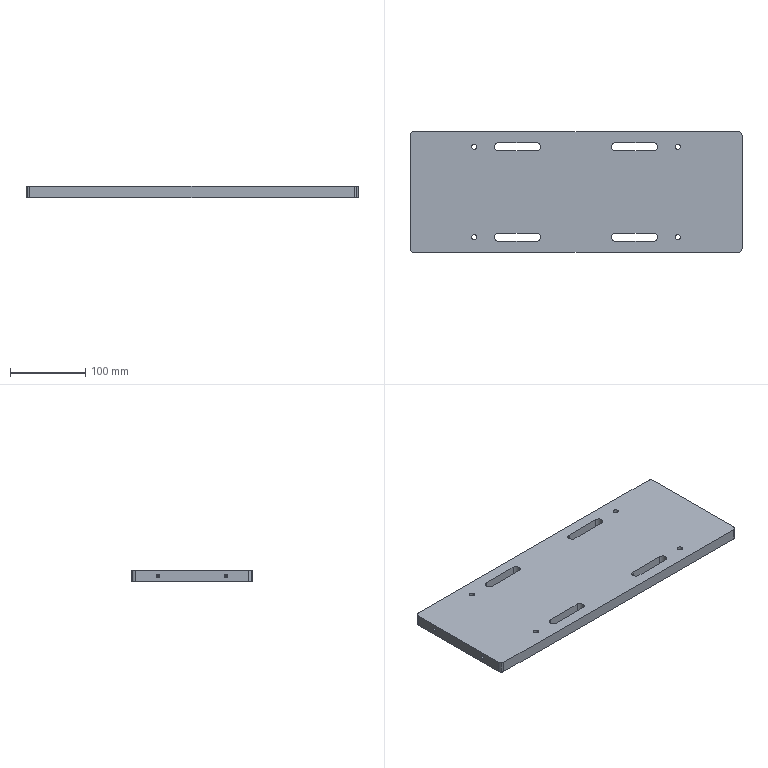Part | STEP file | DCV-000-006 | 1 solid | 46 faces | box 440 x 160 x 15 mm | volume 1014226 mm3 | cylinder 28 | plane 14 | cone 4 | commonest cylinder face diameters 6.647 x8 10 x8 11 x8 4.917 x4